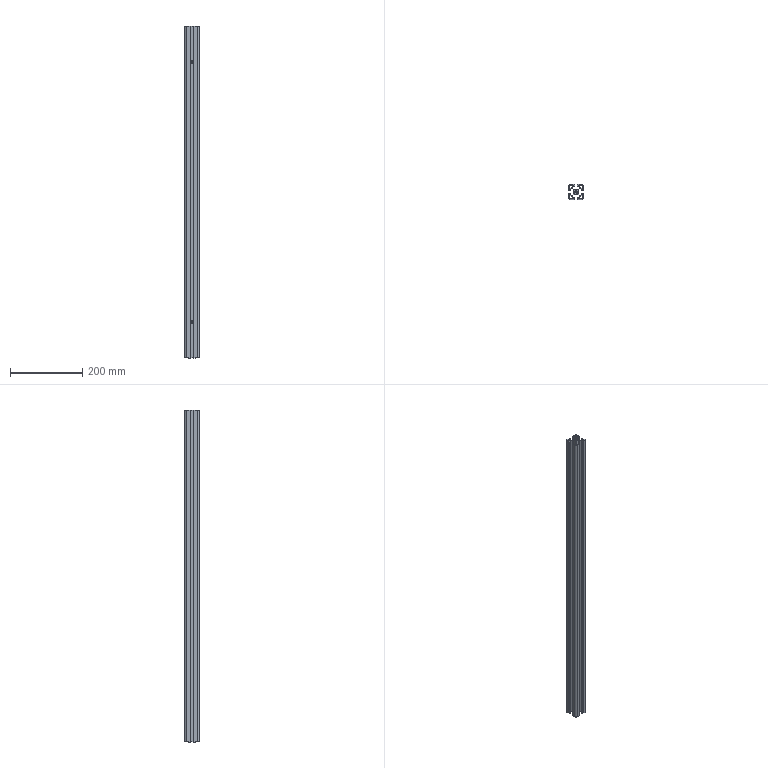Part | STEP file | LE-8-4040-S-OO_LE0311094949 | 1 solid | 228 faces | box 40 x 40 x 920 mm | volume 439466 mm3 | cylinder 122 | plane 106 | commonest cylinder face diameters 0.6 x38 2 x28 4 x16 0.4 x12 6.6 x8 0.458 x6